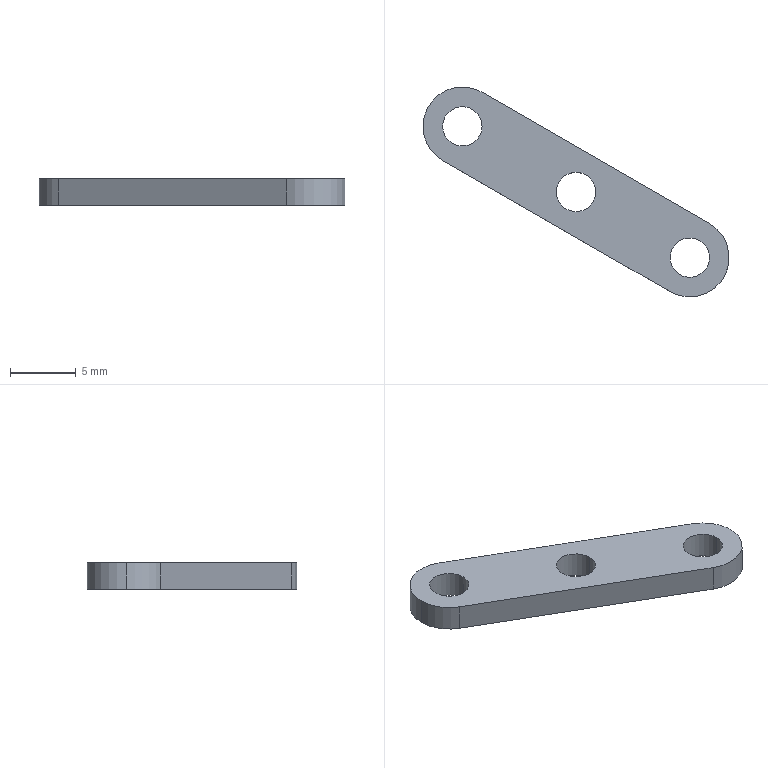Part | SolidWorks | features Extrusion 1 | 1 solid | 13 faces | box 23.321 x 16 x 2 mm | volume 254.137 mm3 | cylinder 9 | plane 4 | commonest cylinder face diameters 3 x6 6 x3
STEP:
#1=CARTESIAN_POINT('',(-10.16,5.,2.));
#2=VERTEX_POINT('',#1);
#3=CARTESIAN_POINT('',(-7.16,5.,2.));
#4=VERTEX_POINT('',#3);
#5=CARTESIAN_POINT('',(-8.66,5.,2.));
#6=DIRECTION('',(0.,0.,1.));
#7=DIRECTION('',(1.,0.,0.));
#8=AXIS2_PLACEMENT_3D('',#5,#6,#7);
#9=CIRCLE('',#8,1.5);
#10=EDGE_CURVE('',#2,#4,#9,.T.);
#11=ORIENTED_EDGE('',*,*,#10,.T.);
#12=CARTESIAN_POINT('',(-7.16,5.,0.));
#13=VERTEX_POINT('',#12);
#14=CARTESIAN_POINT('',(-7.16,5.,2.));
#15=DIRECTION('',(0.,0.,-1.));
#16=VECTOR('',#15,1000.);
#17=LINE('',#14,#16);
#18=EDGE_CURVE('',#4,#13,#17,.T.);
#19=ORIENTED_EDGE('',*,*,#18,.T.);
#20=CARTESIAN_POINT('',(-10.16,5.,0.));
#21=VERTEX_POINT('',#20);
#22=CARTESIAN_POINT('',(-8.66,5.,0.));
#23=DIRECTION('',(0.,0.,1.));
#24=DIRECTION('',(1.,0.,0.));
#25=AXIS2_PLACEMENT_3D('',#22,#23,#24);
#26=CIRCLE('',#25,1.5);
#27=EDGE_CURVE('',#21,#13,#26,.T.);
#28=ORIENTED_EDGE('',*,*,#27,.F.);
#29=CARTESIAN_POINT('',(-10.16,5.,2.));
#30=DIRECTION('',(0.,0.,-1.));
#31=VECTOR('',#30,1000.);
#32=LINE('',#29,#31);
#33=EDGE_CURVE('',#2,#21,#32,.T.);
#34=ORIENTED_EDGE('',*,*,#33,.F.);
#35=EDGE_LOOP('',(#11,#19,#28,#34));
#36=FACE_OUTER_BOUND('',#35,.T.);
#37=CARTESIAN_POINT('',(-8.66,5.,2.));
#38=DIRECTION('',(0.,0.,-1.));
#39=DIRECTION('',(-1.,0.,0.));
#40=AXIS2_PLACEMENT_3D('',#37,#38,#39);
#41=CYLINDRICAL_SURFACE('',#40,1.5);
#42=ADVANCED_FACE('',(#36),#41,.F.);
#43=CARTESIAN_POINT('',(7.16,-5.,2.));
#44=VERTEX_POINT('',#43);
#45=CARTESIAN_POINT('',(10.16,-5.,2.));
#46=VERTEX_POINT('',#45);
#47=CARTESIAN_POINT('',(8.66,-5.,2.));
#48=DIRECTION('',(0.,0.,1.));
#49=DIRECTION('',(1.,0.,0.));
#50=AXIS2_PLACEMENT_3D('',#47,#48,#49);
#51=CIRCLE('',#50,1.5);
#52=EDGE_CURVE('',#44,#46,#51,.T.);
#53=ORIENTED_EDGE('',*,*,#52,.T.);
#54=CARTESIAN_POINT('',(10.16,-5.,0.));
#55=VERTEX_POINT('',#54);
#56=CARTESIAN_POINT('',(10.16,-5.,2.));
#57=DIRECTION('',(0.,0.,-1.));
#58=VECTOR('',#57,1000.);
#59=LINE('',#56,#58);
#60=EDGE_CURVE('',#46,#55,#59,.T.);
#61=ORIENTED_EDGE('',*,*,#60,.T.);
#62=CARTESIAN_POINT('',(7.16,-5.,0.));
#63=VERTEX_POINT('',#62);
#64=CARTESIAN_POINT('',(8.66,-5.,0.));
#65=DIRECTION('',(0.,0.,1.));
#66=DIRECTION('',(1.,0.,0.));
#67=AXIS2_PLACEMENT_3D('',#64,#65,#66);
#68=CIRCLE('',#67,1.5);
#69=EDGE_CURVE('',#63,#55,#68,.T.);
#70=ORIENTED_EDGE('',*,*,#69,.F.);
#71=CARTESIAN_POINT('',(7.16,-5.,2.));
#72=DIRECTION('',(0.,0.,-1.));
#73=VECTOR('',#72,1000.);
#74=LINE('',#71,#73);
#75=EDGE_CURVE('',#44,#63,#74,.T.);
#76=ORIENTED_EDGE('',*,*,#75,.F.);
#77=EDGE_LOOP('',(#53,#61,#70,#76));
#78=FACE_OUTER_BOUND('',#77,.T.);
#79=CARTESIAN_POINT('',(8.66,-5.,2.));
#80=DIRECTION('',(0.,0.,-1.));
#81=DIRECTION('',(-1.,0.,0.));
#82=AXIS2_PLACEMENT_3D('',#79,#80,#81);
#83=CYLINDRICAL_SURFACE('',#82,1.5);
#84=ADVANCED_FACE('',(#78),#83,.F.);
#85=CARTESIAN_POINT('',(-1.5,0.,2.));
#86=VERTEX_POINT('',#85);
#87=CARTESIAN_POINT('',(1.5,0.,2.));
#88=VERTEX_POINT('',#87);
#89=CARTESIAN_POINT('',(0.,0.,2.));
#90=DIRECTION('',(0.,0.,1.));
#91=DIRECTION('',(1.,0.,0.));
#92=AXIS2_PLACEMENT_3D('',#89,#90,#91);
#93=CIRCLE('',#92,1.5);
#94=EDGE_CURVE('',#86,#88,#93,.T.);
#95=ORIENTED_EDGE('',*,*,#94,.T.);
#96=CARTESIAN_POINT('',(1.5,0.,0.));
#97=VERTEX_POINT('',#96);
#98=CARTESIAN_POINT('',(1.5,0.,2.));
#99=DIRECTION('',(0.,0.,-1.));
#100=VECTOR('',#99,1000.);
#101=LINE('',#98,#100);
#102=EDGE_CURVE('',#88,#97,#101,.T.);
#103=ORIENTED_EDGE('',*,*,#102,.T.);
#104=CARTESIAN_POINT('',(-1.5,0.,0.));
#105=VERTEX_POINT('',#104);
#106=CARTESIAN_POINT('',(0.,0.,0.));
#107=DIRECTION('',(0.,0.,1.));
#108=DIRECTION('',(1.,0.,0.));
#109=AXIS2_PLACEMENT_3D('',#106,#107,#108);
#110=CIRCLE('',#109,1.5);
#111=EDGE_CURVE('',#105,#97,#110,.T.);
#112=ORIENTED_EDGE('',*,*,#111,.F.);
#113=CARTESIAN_POINT('',(-1.5,0.,2.));
#114=DIRECTION('',(0.,0.,-1.));
#115=VECTOR('',#114,1000.);
#116=LINE('',#113,#115);
#117=EDGE_CURVE('',#86,#105,#116,.T.);
#118=ORIENTED_EDGE('',*,*,#117,.F.);
#119=EDGE_LOOP('',(#95,#103,#112,#118));
#120=FACE_OUTER_BOUND('',#119,.T.);
#121=CARTESIAN_POINT('',(0.,0.,2.));
#122=DIRECTION('',(0.,0.,-1.));
#123=DIRECTION('',(-1.,0.,0.));
#124=AXIS2_PLACEMENT_3D('',#121,#122,#123);
#125=CYLINDRICAL_SURFACE('',#124,1.5);
#126=ADVANCED_FACE('',(#120),#125,.F.);
#127=CARTESIAN_POINT('',(-11.66,5.,2.));
#128=VERTEX_POINT('',#127);
#129=CARTESIAN_POINT('',(-10.16,2.402,2.));
#130=VERTEX_POINT('',#129);
#131=CARTESIAN_POINT('',(-8.66,5.,2.));
#132=DIRECTION('',(0.,0.,1.));
#133=DIRECTION('',(1.,0.,0.));
#134=AXIS2_PLACEMENT_3D('',#131,#132,#133);
#135=CIRCLE('',#134,3.);
#136=EDGE_CURVE('',#128,#130,#135,.T.);
#137=ORIENTED_EDGE('',*,*,#136,.F.);
#138=CARTESIAN_POINT('',(-11.66,5.,0.));
#139=VERTEX_POINT('',#138);
#140=CARTESIAN_POINT('',(-11.66,5.,2.));
#141=DIRECTION('',(0.,0.,-1.));
#142=VECTOR('',#141,1000.);
#143=LINE('',#140,#142);
#144=EDGE_CURVE('',#128,#139,#143,.T.);
#145=ORIENTED_EDGE('',*,*,#144,.T.);
#146=CARTESIAN_POINT('',(-10.16,2.402,0.));
#147=VERTEX_POINT('',#146);
#148=CARTESIAN_POINT('',(-8.66,5.,0.));
#149=DIRECTION('',(0.,0.,1.));
#150=DIRECTION('',(1.,0.,0.));
#151=AXIS2_PLACEMENT_3D('',#148,#149,#150);
#152=CIRCLE('',#151,3.);
#153=EDGE_CURVE('',#139,#147,#152,.T.);
#154=ORIENTED_EDGE('',*,*,#153,.T.);
#155=CARTESIAN_POINT('',(-10.16,2.402,2.));
#156=DIRECTION('',(0.,0.,-1.));
#157=VECTOR('',#156,1000.);
#158=LINE('',#155,#157);
#159=EDGE_CURVE('',#130,#147,#158,.T.);
#160=ORIENTED_EDGE('',*,*,#159,.F.);
#161=EDGE_LOOP('',(#137,#145,#154,#160));
#162=FACE_OUTER_BOUND('',#161,.T.);
#163=CARTESIAN_POINT('',(-8.66,5.,2.));
#164=DIRECTION('',(0.,0.,-1.));
#165=DIRECTION('',(-1.,0.,0.));
#166=AXIS2_PLACEMENT_3D('',#163,#164,#165);
#167=CYLINDRICAL_SURFACE('',#166,3.);
#168=ADVANCED_FACE('',(#162),#167,.T.);
#169=ORIENTED_EDGE('',*,*,#52,.F.);
#170=CARTESIAN_POINT('',(8.66,-5.,2.));
#171=DIRECTION('',(0.,0.,1.));
#172=DIRECTION('',(1.,0.,0.));
#173=AXIS2_PLACEMENT_3D('',#170,#171,#172);
#174=CIRCLE('',#173,1.5);
#175=EDGE_CURVE('',#46,#44,#174,.T.);
#176=ORIENTED_EDGE('',*,*,#175,.F.);
#177=EDGE_LOOP('',(#169,#176));
#178=FACE_BOUND('',#177,.T.);
#179=CARTESIAN_POINT('',(-7.16,7.598,2.));
#180=VERTEX_POINT('',#179);
#181=CARTESIAN_POINT('',(-8.66,5.,2.));
#182=DIRECTION('',(0.,0.,1.));
#183=DIRECTION('',(1.,0.,0.));
#184=AXIS2_PLACEMENT_3D('',#181,#182,#183);
#185=CIRCLE('',#184,3.);
#186=EDGE_CURVE('',#180,#128,#185,.T.);
#187=ORIENTED_EDGE('',*,*,#186,.T.);
#188=ORIENTED_EDGE('',*,*,#136,.T.);
#189=CARTESIAN_POINT('',(7.16,-7.598,2.));
#190=VERTEX_POINT('',#189);
#191=CARTESIAN_POINT('',(-10.16,2.402,2.));
#192=DIRECTION('',(0.866,-0.5,0.));
#193=VECTOR('',#192,1000.);
#194=LINE('',#191,#193);
#195=EDGE_CURVE('',#130,#190,#194,.T.);
#196=ORIENTED_EDGE('',*,*,#195,.T.);
#197=CARTESIAN_POINT('',(10.16,-2.402,2.));
#198=VERTEX_POINT('',#197);
#199=CARTESIAN_POINT('',(8.66,-5.,2.));
#200=DIRECTION('',(0.,0.,1.));
#201=DIRECTION('',(1.,0.,0.));
#202=AXIS2_PLACEMENT_3D('',#199,#200,#201);
#203=CIRCLE('',#202,3.);
#204=EDGE_CURVE('',#190,#198,#203,.T.);
#205=ORIENTED_EDGE('',*,*,#204,.T.);
#206=CARTESIAN_POINT('',(-7.16,7.598,2.));
#207=DIRECTION('',(-0.866,0.5,0.));
#208=VECTOR('',#207,1000.);
#209=LINE('',#206,#208);
#210=EDGE_CURVE('',#198,#180,#209,.T.);
#211=ORIENTED_EDGE('',*,*,#210,.T.);
#212=EDGE_LOOP('',(#187,#188,#196,#205,#211));
#213=FACE_OUTER_BOUND('',#212,.T.);
#214=ORIENTED_EDGE('',*,*,#94,.F.);
#215=CARTESIAN_POINT('',(0.,0.,2.));
#216=DIRECTION('',(0.,0.,1.));
#217=DIRECTION('',(1.,0.,0.));
#218=AXIS2_PLACEMENT_3D('',#215,#216,#217);
#219=CIRCLE('',#218,1.5);
#220=EDGE_CURVE('',#88,#86,#219,.T.);
#221=ORIENTED_EDGE('',*,*,#220,.F.);
#222=EDGE_LOOP('',(#214,#221));
#223=FACE_BOUND('',#222,.T.);
#224=ORIENTED_EDGE('',*,*,#10,.F.);
#225=CARTESIAN_POINT('',(-8.66,5.,2.));
#226=DIRECTION('',(0.,0.,1.));
#227=DIRECTION('',(1.,0.,0.));
#228=AXIS2_PLACEMENT_3D('',#225,#226,#227);
#229=CIRCLE('',#228,1.5);
#230=EDGE_CURVE('',#4,#2,#229,.T.);
#231=ORIENTED_EDGE('',*,*,#230,.F.);
#232=EDGE_LOOP('',(#224,#231));
#233=FACE_BOUND('',#232,.T.);
#234=CARTESIAN_POINT('',(-8.66,5.,2.));
#235=DIRECTION('',(0.,0.,1.));
#236=DIRECTION('',(1.,0.,0.));
#237=AXIS2_PLACEMENT_3D('',#234,#235,#236);
#238=PLANE('',#237);
#239=ADVANCED_FACE('',(#178,#213,#223,#233),#238,.T.);
#240=CARTESIAN_POINT('',(-7.16,7.598,0.));
#241=VERTEX_POINT('',#240);
#242=CARTESIAN_POINT('',(-8.66,5.,0.));
#243=DIRECTION('',(0.,0.,1.));
#244=DIRECTION('',(1.,0.,0.));
#245=AXIS2_PLACEMENT_3D('',#242,#243,#244);
#246=CIRCLE('',#245,3.);
#247=EDGE_CURVE('',#241,#139,#246,.T.);
#248=ORIENTED_EDGE('',*,*,#247,.F.);
#249=CARTESIAN_POINT('',(10.16,-2.402,0.));
#250=VERTEX_POINT('',#249);
#251=CARTESIAN_POINT('',(-7.16,7.598,0.));
#252=DIRECTION('',(-0.866,0.5,0.));
#253=VECTOR('',#252,1000.);
#254=LINE('',#251,#253);
#255=EDGE_CURVE('',#250,#241,#254,.T.);
#256=ORIENTED_EDGE('',*,*,#255,.F.);
#257=CARTESIAN_POINT('',(7.16,-7.598,0.));
#258=VERTEX_POINT('',#257);
#259=CARTESIAN_POINT('',(8.66,-5.,0.));
#260=DIRECTION('',(0.,0.,1.));
#261=DIRECTION('',(1.,0.,0.));
#262=AXIS2_PLACEMENT_3D('',#259,#260,#261);
#263=CIRCLE('',#262,3.);
#264=EDGE_CURVE('',#258,#250,#263,.T.);
#265=ORIENTED_EDGE('',*,*,#264,.F.);
#266=CARTESIAN_POINT('',(-10.16,2.402,0.));
#267=DIRECTION('',(0.866,-0.5,0.));
#268=VECTOR('',#267,1000.);
#269=LINE('',#266,#268);
#270=EDGE_CURVE('',#147,#258,#269,.T.);
#271=ORIENTED_EDGE('',*,*,#270,.F.);
#272=ORIENTED_EDGE('',*,*,#153,.F.);
#273=EDGE_LOOP('',(#248,#256,#265,#271,#272));
#274=FACE_OUTER_BOUND('',#273,.T.);
#275=ORIENTED_EDGE('',*,*,#111,.T.);
#276=CARTESIAN_POINT('',(0.,0.,0.));
#277=DIRECTION('',(0.,0.,1.));
#278=DIRECTION('',(1.,0.,0.));
#279=AXIS2_PLACEMENT_3D('',#276,#277,#278);
#280=CIRCLE('',#279,1.5);
#281=EDGE_CURVE('',#97,#105,#280,.T.);
#282=ORIENTED_EDGE('',*,*,#281,.T.);
#283=EDGE_LOOP('',(#275,#282));
#284=FACE_BOUND('',#283,.T.);
#285=ORIENTED_EDGE('',*,*,#69,.T.);
#286=CARTESIAN_POINT('',(8.66,-5.,0.));
#287=DIRECTION('',(0.,0.,1.));
#288=DIRECTION('',(1.,0.,0.));
#289=AXIS2_PLACEMENT_3D('',#286,#287,#288);
#290=CIRCLE('',#289,1.5);
#291=EDGE_CURVE('',#55,#63,#290,.T.);
#292=ORIENTED_EDGE('',*,*,#291,.T.);
#293=EDGE_LOOP('',(#285,#292));
#294=FACE_BOUND('',#293,.T.);
#295=ORIENTED_EDGE('',*,*,#27,.T.);
#296=CARTESIAN_POINT('',(-8.66,5.,0.));
#297=DIRECTION('',(0.,0.,1.));
#298=DIRECTION('',(1.,0.,0.));
#299=AXIS2_PLACEMENT_3D('',#296,#297,#298);
#300=CIRCLE('',#299,1.5);
#301=EDGE_CURVE('',#13,#21,#300,.T.);
#302=ORIENTED_EDGE('',*,*,#301,.T.);
#303=EDGE_LOOP('',(#295,#302));
#304=FACE_BOUND('',#303,.T.);
#305=CARTESIAN_POINT('',(-8.66,5.,0.));
#306=DIRECTION('',(0.,0.,1.));
#307=DIRECTION('',(1.,0.,0.));
#308=AXIS2_PLACEMENT_3D('',#305,#306,#307);
#309=PLANE('',#308);
#310=ADVANCED_FACE('',(#274,#284,#294,#304),#309,.F.);
#311=ORIENTED_EDGE('',*,*,#144,.F.);
#312=ORIENTED_EDGE('',*,*,#186,.F.);
#313=CARTESIAN_POINT('',(-7.16,7.598,2.));
#314=DIRECTION('',(0.,0.,-1.));
#315=VECTOR('',#314,1000.);
#316=LINE('',#313,#315);
#317=EDGE_CURVE('',#180,#241,#316,.T.);
#318=ORIENTED_EDGE('',*,*,#317,.T.);
#319=ORIENTED_EDGE('',*,*,#247,.T.);
#320=EDGE_LOOP('',(#311,#312,#318,#319));
#321=FACE_OUTER_BOUND('',#320,.T.);
#322=CARTESIAN_POINT('',(-8.66,5.,2.));
#323=DIRECTION('',(0.,0.,-1.));
#324=DIRECTION('',(-1.,0.,0.));
#325=AXIS2_PLACEMENT_3D('',#322,#323,#324);
#326=CYLINDRICAL_SURFACE('',#325,3.);
#327=ADVANCED_FACE('',(#321),#326,.T.);
#328=ORIENTED_EDGE('',*,*,#270,.T.);
#329=CARTESIAN_POINT('',(7.16,-7.598,2.));
#330=DIRECTION('',(0.,0.,-1.));
#331=VECTOR('',#330,1000.);
#332=LINE('',#329,#331);
#333=EDGE_CURVE('',#190,#258,#332,.T.);
#334=ORIENTED_EDGE('',*,*,#333,.F.);
#335=ORIENTED_EDGE('',*,*,#195,.F.);
#336=ORIENTED_EDGE('',*,*,#159,.T.);
#337=EDGE_LOOP('',(#328,#334,#335,#336));
#338=FACE_OUTER_BOUND('',#337,.T.);
#339=CARTESIAN_POINT('',(-10.16,2.402,2.));
#340=DIRECTION('',(0.5,0.866,0.));
#341=DIRECTION('',(-0.866,0.5,0.));
#342=AXIS2_PLACEMENT_3D('',#339,#340,#341);
#343=PLANE('',#342);
#344=ADVANCED_FACE('',(#338),#343,.F.);
#345=ORIENTED_EDGE('',*,*,#264,.T.);
#346=CARTESIAN_POINT('',(10.16,-2.402,2.));
#347=DIRECTION('',(0.,0.,-1.));
#348=VECTOR('',#347,1000.);
#349=LINE('',#346,#348);
#350=EDGE_CURVE('',#198,#250,#349,.T.);
#351=ORIENTED_EDGE('',*,*,#350,.F.);
#352=ORIENTED_EDGE('',*,*,#204,.F.);
#353=ORIENTED_EDGE('',*,*,#333,.T.);
#354=EDGE_LOOP('',(#345,#351,#352,#353));
#355=FACE_OUTER_BOUND('',#354,.T.);
#356=CARTESIAN_POINT('',(8.66,-5.,2.));
#357=DIRECTION('',(0.,0.,-1.));
#358=DIRECTION('',(-1.,0.,0.));
#359=AXIS2_PLACEMENT_3D('',#356,#357,#358);
#360=CYLINDRICAL_SURFACE('',#359,3.);
#361=ADVANCED_FACE('',(#355),#360,.T.);
#362=ORIENTED_EDGE('',*,*,#255,.T.);
#363=ORIENTED_EDGE('',*,*,#317,.F.);
#364=ORIENTED_EDGE('',*,*,#210,.F.);
#365=ORIENTED_EDGE('',*,*,#350,.T.);
#366=EDGE_LOOP('',(#362,#363,#364,#365));
#367=FACE_OUTER_BOUND('',#366,.T.);
#368=CARTESIAN_POINT('',(-7.16,7.598,2.));
#369=DIRECTION('',(-0.5,-0.866,0.));
#370=DIRECTION('',(0.866,-0.5,0.));
#371=AXIS2_PLACEMENT_3D('',#368,#369,#370);
#372=PLANE('',#371);
#373=ADVANCED_FACE('',(#367),#372,.F.);
#374=ORIENTED_EDGE('',*,*,#102,.F.);
#375=ORIENTED_EDGE('',*,*,#220,.T.);
#376=ORIENTED_EDGE('',*,*,#117,.T.);
#377=ORIENTED_EDGE('',*,*,#281,.F.);
#378=EDGE_LOOP('',(#374,#375,#376,#377));
#379=FACE_OUTER_BOUND('',#378,.T.);
#380=CARTESIAN_POINT('',(0.,0.,2.));
#381=DIRECTION('',(0.,0.,-1.));
#382=DIRECTION('',(-1.,0.,0.));
#383=AXIS2_PLACEMENT_3D('',#380,#381,#382);
#384=CYLINDRICAL_SURFACE('',#383,1.5);
#385=ADVANCED_FACE('',(#379),#384,.F.);
#386=ORIENTED_EDGE('',*,*,#60,.F.);
#387=ORIENTED_EDGE('',*,*,#175,.T.);
#388=ORIENTED_EDGE('',*,*,#75,.T.);
#389=ORIENTED_EDGE('',*,*,#291,.F.);
#390=EDGE_LOOP('',(#386,#387,#388,#389));
#391=FACE_OUTER_BOUND('',#390,.T.);
#392=CARTESIAN_POINT('',(8.66,-5.,2.));
#393=DIRECTION('',(0.,0.,-1.));
#394=DIRECTION('',(-1.,0.,0.));
#395=AXIS2_PLACEMENT_3D('',#392,#393,#394);
#396=CYLINDRICAL_SURFACE('',#395,1.5);
#397=ADVANCED_FACE('',(#391),#396,.F.);
#398=ORIENTED_EDGE('',*,*,#18,.F.);
#399=ORIENTED_EDGE('',*,*,#230,.T.);
#400=ORIENTED_EDGE('',*,*,#33,.T.);
#401=ORIENTED_EDGE('',*,*,#301,.F.);
#402=EDGE_LOOP('',(#398,#399,#400,#401));
#403=FACE_OUTER_BOUND('',#402,.T.);
#404=CARTESIAN_POINT('',(-8.66,5.,2.));
#405=DIRECTION('',(0.,0.,-1.));
#406=DIRECTION('',(-1.,0.,0.));
#407=AXIS2_PLACEMENT_3D('',#404,#405,#406);
#408=CYLINDRICAL_SURFACE('',#407,1.5);
#409=ADVANCED_FACE('',(#403),#408,.F.);
#410=CLOSED_SHELL('',(#42,#84,#126,#168,#239,#310,#327,#344,#361,#373,#385,#397,#409));
#411=MANIFOLD_SOLID_BREP('',#410);
#412=CARTESIAN_POINT('',(0.,0.,0.));
#413=DIRECTION('',(0.,0.,1.));
#414=DIRECTION('',(1.,0.,0.));
#415=AXIS2_PLACEMENT_3D('',#412,#413,#414);
#416=(LENGTH_UNIT()NAMED_UNIT(*)SI_UNIT(.MILLI.,.METRE.));
#417=UNCERTAINTY_MEASURE_WITH_UNIT(LENGTH_MEASURE(0.00001),#416,'','');
#418=(NAMED_UNIT(*)PLANE_ANGLE_UNIT()SI_UNIT($,.RADIAN.));
#419=(NAMED_UNIT(*)SI_UNIT($,.STERADIAN.)SOLID_ANGLE_UNIT());
#420=(GEOMETRIC_REPRESENTATION_CONTEXT(3)GLOBAL_UNCERTAINTY_ASSIGNED_CONTEXT((#417))GLOBAL_UNIT_ASSIGNED_CONTEXT((#416,#418,#419))REPRESENTATION_CONTEXT('',''));
#421=ADVANCED_BREP_SHAPE_REPRESENTATION('',(#411,#415),#420);